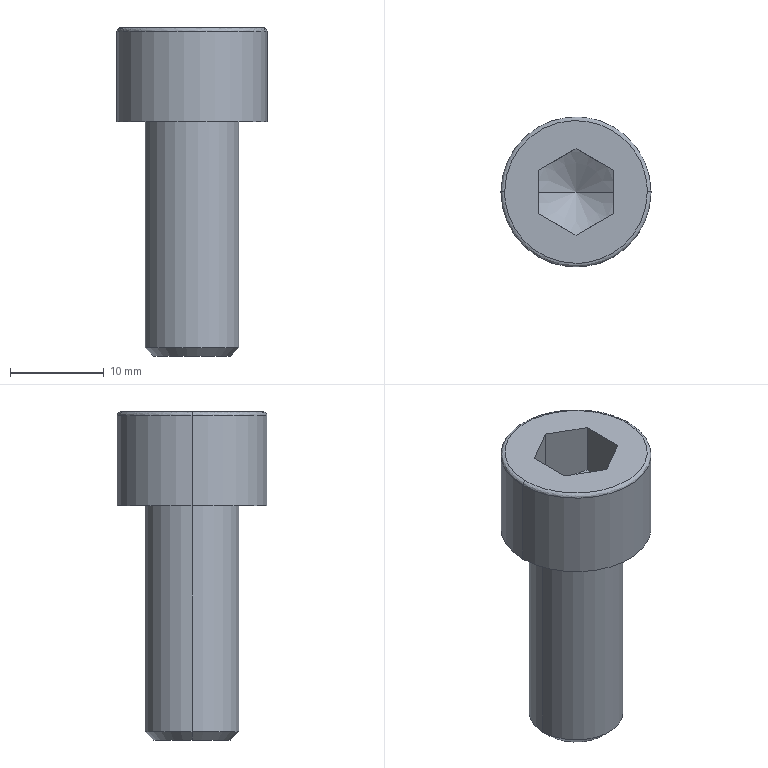Part | STEP file | 45 | 1 solid | 19 faces | box 16 x 16 x 35 mm | volume 3597 mm3 | plane 9 | cylinder 4 | cone 4 | spline 2 | commonest cylinder face diameters 10 x2 16 x2